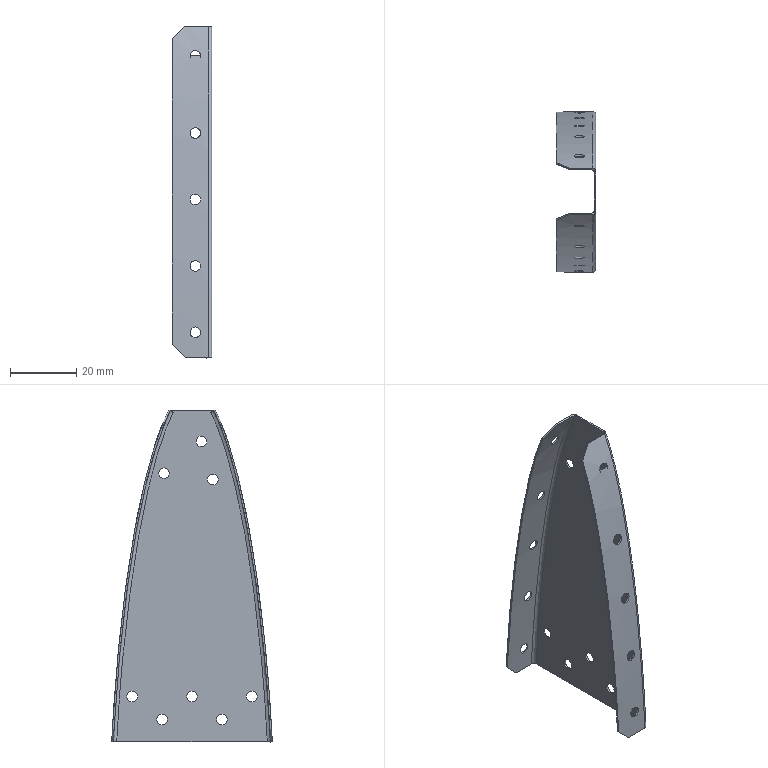Part | SolidWorks | features BaseBody 1 | 1 solid | 56 faces | box 12 x 48.392 x 100 mm | volume 2919 mm3 | cylinder 35 | plane 13 | spline 8 | commonest cylinder face diameters 3.2 x35